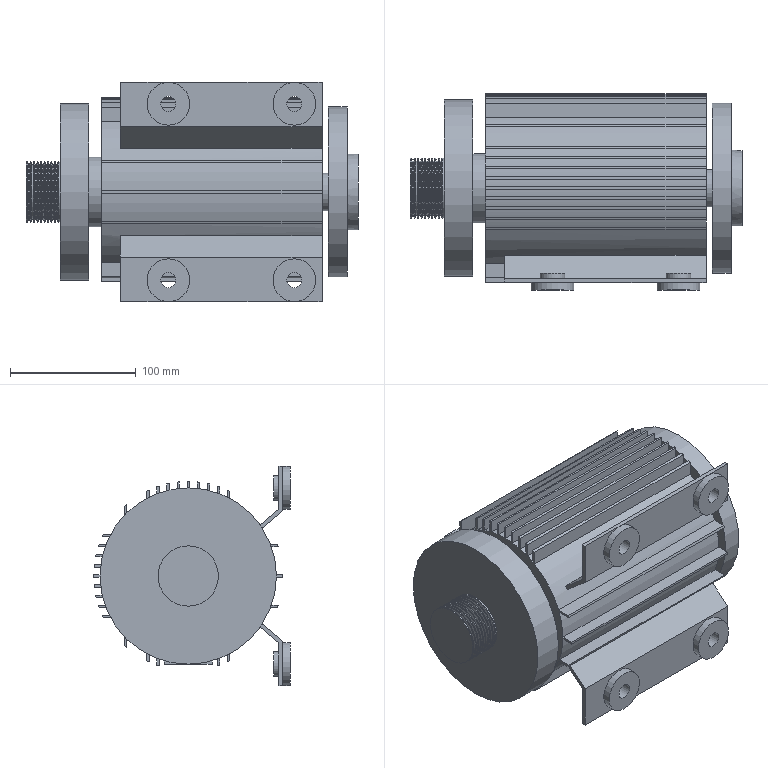Part | STEP file | AC MOTOR 1.5KW | 1 solid | 303 faces | box 263.5 x 156.005 x 174 mm | volume 3095920 mm3 | cylinder 130 | plane 128 | torus 27 | cone 18 | commonest cylinder face diameters 2 x32 130 x27 150.011 x27 100 x9 125 x8 12 x4